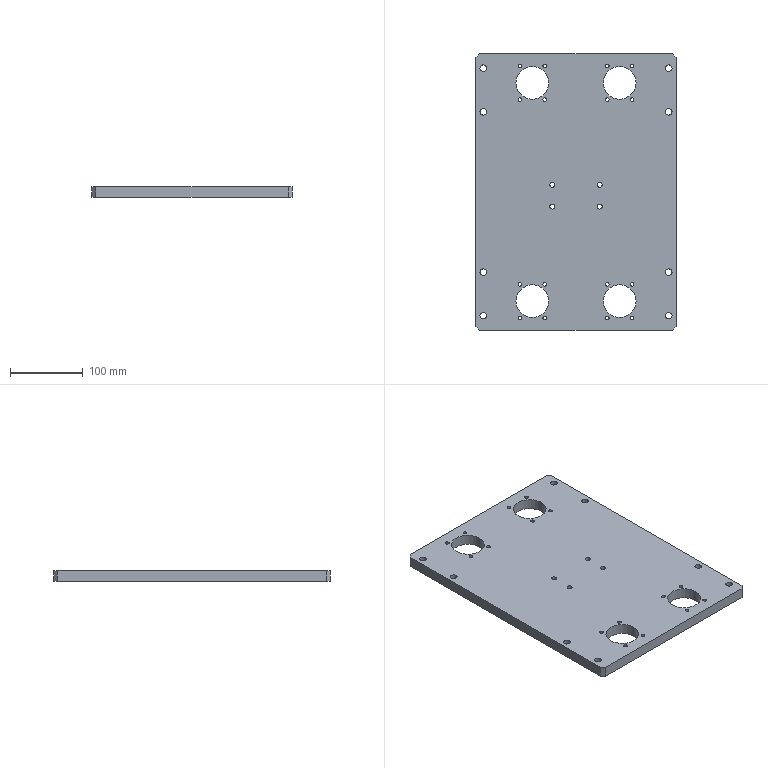Part | SolidWorks | features BaseBody 1 | 1 solid | 98 faces | box 275 x 380 x 15 mm | volume 1449018 mm3 | cylinder 80 | plane 18 | commonest cylinder face diameters 5 x32 9 x16 15 x16 6.8 x8 45 x8